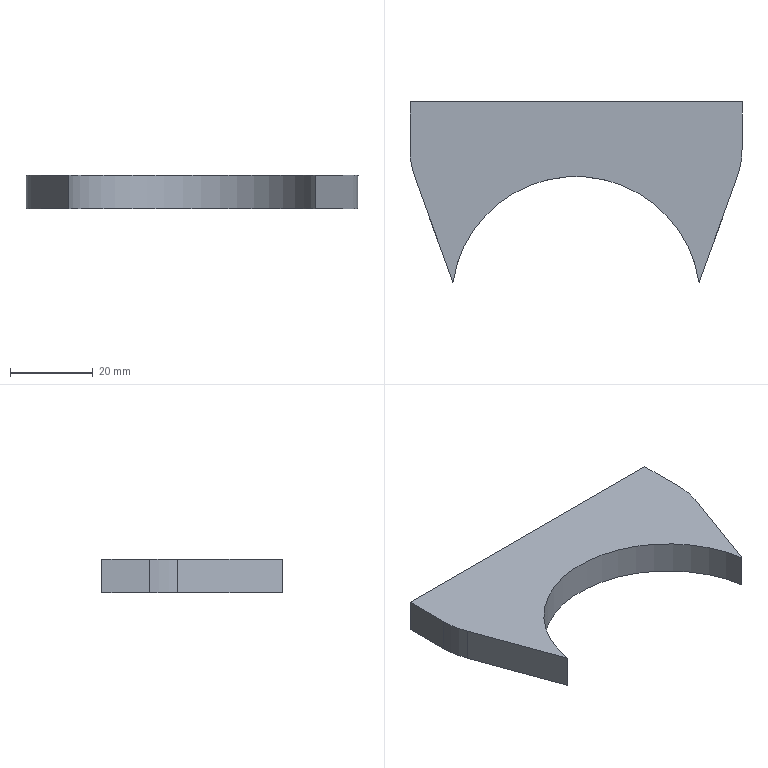Part | SolidWorks | features Fillet 1, FlatPattern 1, SMBaseFlange 1, SheetMetal 1 | 1 solid | 10 faces | box 80 x 43.435 x 8 mm | volume 16306 mm3 | plane 7 | cylinder 3 | commonest cylinder face diameters 40 x2 60 x1
STEP:
#1=CARTESIAN_POINT('',(-40.,48.,-8.));
#2=VERTEX_POINT('',#1);
#3=CARTESIAN_POINT('',(-40.,36.527,-8.));
#4=VERTEX_POINT('',#3);
#5=CARTESIAN_POINT('',(-40.,48.,-8.));
#6=DIRECTION('',(0.,-1.,0.));
#7=VECTOR('',#6,1000.);
#8=LINE('',#5,#7);
#9=EDGE_CURVE('',#2,#4,#8,.T.);
#10=ORIENTED_EDGE('',*,*,#9,.T.);
#11=CARTESIAN_POINT('',(-40.,36.527,0.));
#12=VERTEX_POINT('',#11);
#13=CARTESIAN_POINT('',(-40.,36.527,-8.));
#14=DIRECTION('',(0.,0.,1.));
#15=VECTOR('',#14,1000.);
#16=LINE('',#13,#15);
#17=EDGE_CURVE('',#4,#12,#16,.T.);
#18=ORIENTED_EDGE('',*,*,#17,.T.);
#19=CARTESIAN_POINT('',(-40.,48.,0.));
#20=VERTEX_POINT('',#19);
#21=CARTESIAN_POINT('',(-40.,48.,0.));
#22=DIRECTION('',(0.,-1.,0.));
#23=VECTOR('',#22,1000.);
#24=LINE('',#21,#23);
#25=EDGE_CURVE('',#20,#12,#24,.T.);
#26=ORIENTED_EDGE('',*,*,#25,.F.);
#27=CARTESIAN_POINT('',(-40.,48.,-8.));
#28=DIRECTION('',(0.,0.,1.));
#29=VECTOR('',#28,1000.);
#30=LINE('',#27,#29);
#31=EDGE_CURVE('',#2,#20,#30,.T.);
#32=ORIENTED_EDGE('',*,*,#31,.F.);
#33=EDGE_LOOP('',(#10,#18,#26,#32));
#34=FACE_OUTER_BOUND('',#33,.T.);
#35=CARTESIAN_POINT('',(-40.,48.,-8.));
#36=DIRECTION('',(-1.,0.,0.));
#37=DIRECTION('',(0.,-1.,0.));
#38=AXIS2_PLACEMENT_3D('',#35,#36,#37);
#39=PLANE('',#38);
#40=ADVANCED_FACE('',(#34),#39,.T.);
#41=CARTESIAN_POINT('',(40.,48.,0.));
#42=VERTEX_POINT('',#41);
#43=CARTESIAN_POINT('',(-40.,48.,0.));
#44=DIRECTION('',(-1.,0.,0.));
#45=VECTOR('',#44,1000.);
#46=LINE('',#43,#45);
#47=EDGE_CURVE('',#42,#20,#46,.T.);
#48=ORIENTED_EDGE('',*,*,#47,.F.);
#49=CARTESIAN_POINT('',(40.,48.,-8.));
#50=VERTEX_POINT('',#49);
#51=CARTESIAN_POINT('',(40.,48.,-8.));
#52=DIRECTION('',(0.,0.,1.));
#53=VECTOR('',#52,1000.);
#54=LINE('',#51,#53);
#55=EDGE_CURVE('',#50,#42,#54,.T.);
#56=ORIENTED_EDGE('',*,*,#55,.F.);
#57=CARTESIAN_POINT('',(-40.,48.,-8.));
#58=DIRECTION('',(-1.,0.,0.));
#59=VECTOR('',#58,1000.);
#60=LINE('',#57,#59);
#61=EDGE_CURVE('',#50,#2,#60,.T.);
#62=ORIENTED_EDGE('',*,*,#61,.T.);
#63=ORIENTED_EDGE('',*,*,#31,.T.);
#64=EDGE_LOOP('',(#48,#56,#62,#63));
#65=FACE_OUTER_BOUND('',#64,.T.);
#66=CARTESIAN_POINT('',(-40.,48.,-8.));
#67=DIRECTION('',(0.,1.,0.));
#68=DIRECTION('',(-1.,0.,0.));
#69=AXIS2_PLACEMENT_3D('',#66,#67,#68);
#70=PLANE('',#69);
#71=ADVANCED_FACE('',(#65),#70,.T.);
#72=CARTESIAN_POINT('',(40.,36.527,0.));
#73=VERTEX_POINT('',#72);
#74=CARTESIAN_POINT('',(40.,33.,0.));
#75=DIRECTION('',(0.,1.,0.));
#76=VECTOR('',#75,1000.);
#77=LINE('',#74,#76);
#78=EDGE_CURVE('',#73,#42,#77,.T.);
#79=ORIENTED_EDGE('',*,*,#78,.F.);
#80=CARTESIAN_POINT('',(40.,36.527,-8.));
#81=VERTEX_POINT('',#80);
#82=CARTESIAN_POINT('',(40.,36.527,-8.));
#83=DIRECTION('',(0.,0.,-1.));
#84=VECTOR('',#83,1000.);
#85=LINE('',#82,#84);
#86=EDGE_CURVE('',#73,#81,#85,.T.);
#87=ORIENTED_EDGE('',*,*,#86,.T.);
#88=CARTESIAN_POINT('',(40.,33.,-8.));
#89=DIRECTION('',(0.,1.,0.));
#90=VECTOR('',#89,1000.);
#91=LINE('',#88,#90);
#92=EDGE_CURVE('',#81,#50,#91,.T.);
#93=ORIENTED_EDGE('',*,*,#92,.T.);
#94=ORIENTED_EDGE('',*,*,#55,.T.);
#95=EDGE_LOOP('',(#79,#87,#93,#94));
#96=FACE_OUTER_BOUND('',#95,.T.);
#97=CARTESIAN_POINT('',(40.,33.,-8.));
#98=DIRECTION('',(1.,0.,0.));
#99=DIRECTION('',(0.,1.,0.));
#100=AXIS2_PLACEMENT_3D('',#97,#98,#99);
#101=PLANE('',#100);
#102=ADVANCED_FACE('',(#96),#101,.T.);
#103=CARTESIAN_POINT('',(29.651,4.565,-8.));
#104=VERTEX_POINT('',#103);
#105=CARTESIAN_POINT('',(38.794,29.686,-8.));
#106=VERTEX_POINT('',#105);
#107=CARTESIAN_POINT('',(29.651,4.565,-8.));
#108=DIRECTION('',(0.342,0.9397,0.));
#109=VECTOR('',#108,1000.);
#110=LINE('',#107,#109);
#111=EDGE_CURVE('',#104,#106,#110,.T.);
#112=ORIENTED_EDGE('',*,*,#111,.T.);
#113=CARTESIAN_POINT('',(38.794,29.686,0.));
#114=VERTEX_POINT('',#113);
#115=CARTESIAN_POINT('',(38.794,29.686,-8.));
#116=DIRECTION('',(0.,0.,1.));
#117=VECTOR('',#116,1000.);
#118=LINE('',#115,#117);
#119=EDGE_CURVE('',#106,#114,#118,.T.);
#120=ORIENTED_EDGE('',*,*,#119,.T.);
#121=CARTESIAN_POINT('',(29.651,4.565,0.));
#122=VERTEX_POINT('',#121);
#123=CARTESIAN_POINT('',(29.651,4.565,0.));
#124=DIRECTION('',(0.342,0.9397,0.));
#125=VECTOR('',#124,1000.);
#126=LINE('',#123,#125);
#127=EDGE_CURVE('',#122,#114,#126,.T.);
#128=ORIENTED_EDGE('',*,*,#127,.F.);
#129=CARTESIAN_POINT('',(29.651,4.565,-8.));
#130=DIRECTION('',(0.,0.,1.));
#131=VECTOR('',#130,1000.);
#132=LINE('',#129,#131);
#133=EDGE_CURVE('',#104,#122,#132,.T.);
#134=ORIENTED_EDGE('',*,*,#133,.F.);
#135=EDGE_LOOP('',(#112,#120,#128,#134));
#136=FACE_OUTER_BOUND('',#135,.T.);
#137=CARTESIAN_POINT('',(29.651,4.565,-8.));
#138=DIRECTION('',(0.9397,-0.342,0.));
#139=DIRECTION('',(0.342,0.9397,0.));
#140=AXIS2_PLACEMENT_3D('',#137,#138,#139);
#141=PLANE('',#140);
#142=ADVANCED_FACE('',(#136),#141,.T.);
#143=CARTESIAN_POINT('',(-29.651,4.565,0.));
#144=VERTEX_POINT('',#143);
#145=CARTESIAN_POINT('',(0.,0.,0.));
#146=DIRECTION('',(0.,0.,-1.));
#147=DIRECTION('',(1.,0.,0.));
#148=AXIS2_PLACEMENT_3D('',#145,#146,#147);
#149=CIRCLE('',#148,30.);
#150=EDGE_CURVE('',#144,#122,#149,.T.);
#151=ORIENTED_EDGE('',*,*,#150,.F.);
#152=CARTESIAN_POINT('',(-29.651,4.565,-8.));
#153=VERTEX_POINT('',#152);
#154=CARTESIAN_POINT('',(-29.651,4.565,-8.));
#155=DIRECTION('',(0.,0.,1.));
#156=VECTOR('',#155,1000.);
#157=LINE('',#154,#156);
#158=EDGE_CURVE('',#153,#144,#157,.T.);
#159=ORIENTED_EDGE('',*,*,#158,.F.);
#160=CARTESIAN_POINT('',(0.,0.,-8.));
#161=DIRECTION('',(0.,0.,-1.));
#162=DIRECTION('',(1.,0.,0.));
#163=AXIS2_PLACEMENT_3D('',#160,#161,#162);
#164=CIRCLE('',#163,30.);
#165=EDGE_CURVE('',#153,#104,#164,.T.);
#166=ORIENTED_EDGE('',*,*,#165,.T.);
#167=ORIENTED_EDGE('',*,*,#133,.T.);
#168=EDGE_LOOP('',(#151,#159,#166,#167));
#169=FACE_OUTER_BOUND('',#168,.T.);
#170=CARTESIAN_POINT('',(0.,0.,-8.));
#171=DIRECTION('',(0.,0.,1.));
#172=DIRECTION('',(1.,0.,0.));
#173=AXIS2_PLACEMENT_3D('',#170,#171,#172);
#174=CYLINDRICAL_SURFACE('',#173,30.);
#175=ADVANCED_FACE('',(#169),#174,.F.);
#176=CARTESIAN_POINT('',(-38.794,29.686,0.));
#177=VERTEX_POINT('',#176);
#178=CARTESIAN_POINT('',(-40.,33.,0.));
#179=DIRECTION('',(0.342,-0.9397,0.));
#180=VECTOR('',#179,1000.);
#181=LINE('',#178,#180);
#182=EDGE_CURVE('',#177,#144,#181,.T.);
#183=ORIENTED_EDGE('',*,*,#182,.F.);
#184=CARTESIAN_POINT('',(-38.794,29.686,-8.));
#185=VERTEX_POINT('',#184);
#186=CARTESIAN_POINT('',(-38.794,29.686,-8.));
#187=DIRECTION('',(0.,0.,-1.));
#188=VECTOR('',#187,1000.);
#189=LINE('',#186,#188);
#190=EDGE_CURVE('',#177,#185,#189,.T.);
#191=ORIENTED_EDGE('',*,*,#190,.T.);
#192=CARTESIAN_POINT('',(-40.,33.,-8.));
#193=DIRECTION('',(0.342,-0.9397,0.));
#194=VECTOR('',#193,1000.);
#195=LINE('',#192,#194);
#196=EDGE_CURVE('',#185,#153,#195,.T.);
#197=ORIENTED_EDGE('',*,*,#196,.T.);
#198=ORIENTED_EDGE('',*,*,#158,.T.);
#199=EDGE_LOOP('',(#183,#191,#197,#198));
#200=FACE_OUTER_BOUND('',#199,.T.);
#201=CARTESIAN_POINT('',(-40.,33.,-8.));
#202=DIRECTION('',(-0.9397,-0.342,0.));
#203=DIRECTION('',(0.342,-0.9397,0.));
#204=AXIS2_PLACEMENT_3D('',#201,#202,#203);
#205=PLANE('',#204);
#206=ADVANCED_FACE('',(#200),#205,.T.);
#207=ORIENTED_EDGE('',*,*,#92,.F.);
#208=CARTESIAN_POINT('',(20.,36.527,-8.));
#209=DIRECTION('',(0.,0.,-1.));
#210=DIRECTION('',(1.,0.,0.));
#211=AXIS2_PLACEMENT_3D('',#208,#209,#210);
#212=CIRCLE('',#211,20.);
#213=EDGE_CURVE('',#81,#106,#212,.T.);
#214=ORIENTED_EDGE('',*,*,#213,.T.);
#215=ORIENTED_EDGE('',*,*,#111,.F.);
#216=ORIENTED_EDGE('',*,*,#165,.F.);
#217=ORIENTED_EDGE('',*,*,#196,.F.);
#218=CARTESIAN_POINT('',(-20.,36.527,-8.));
#219=DIRECTION('',(0.,0.,-1.));
#220=DIRECTION('',(1.,0.,0.));
#221=AXIS2_PLACEMENT_3D('',#218,#219,#220);
#222=CIRCLE('',#221,20.);
#223=EDGE_CURVE('',#185,#4,#222,.T.);
#224=ORIENTED_EDGE('',*,*,#223,.T.);
#225=ORIENTED_EDGE('',*,*,#9,.F.);
#226=ORIENTED_EDGE('',*,*,#61,.F.);
#227=EDGE_LOOP('',(#207,#214,#215,#216,#217,#224,#225,#226));
#228=FACE_OUTER_BOUND('',#227,.T.);
#229=CARTESIAN_POINT('',(0.,0.,-8.));
#230=DIRECTION('',(0.,0.,1.));
#231=DIRECTION('',(1.,0.,0.));
#232=AXIS2_PLACEMENT_3D('',#229,#230,#231);
#233=PLANE('',#232);
#234=ADVANCED_FACE('',(#228),#233,.F.);
#235=ORIENTED_EDGE('',*,*,#127,.T.);
#236=CARTESIAN_POINT('',(20.,36.527,0.));
#237=DIRECTION('',(0.,0.,1.));
#238=DIRECTION('',(1.,0.,0.));
#239=AXIS2_PLACEMENT_3D('',#236,#237,#238);
#240=CIRCLE('',#239,20.);
#241=EDGE_CURVE('',#114,#73,#240,.T.);
#242=ORIENTED_EDGE('',*,*,#241,.T.);
#243=ORIENTED_EDGE('',*,*,#78,.T.);
#244=ORIENTED_EDGE('',*,*,#47,.T.);
#245=ORIENTED_EDGE('',*,*,#25,.T.);
#246=CARTESIAN_POINT('',(-20.,36.527,0.));
#247=DIRECTION('',(0.,0.,1.));
#248=DIRECTION('',(1.,0.,0.));
#249=AXIS2_PLACEMENT_3D('',#246,#247,#248);
#250=CIRCLE('',#249,20.);
#251=EDGE_CURVE('',#12,#177,#250,.T.);
#252=ORIENTED_EDGE('',*,*,#251,.T.);
#253=ORIENTED_EDGE('',*,*,#182,.T.);
#254=ORIENTED_EDGE('',*,*,#150,.T.);
#255=EDGE_LOOP('',(#235,#242,#243,#244,#245,#252,#253,#254));
#256=FACE_OUTER_BOUND('',#255,.T.);
#257=CARTESIAN_POINT('',(0.,0.,0.));
#258=DIRECTION('',(0.,0.,1.));
#259=DIRECTION('',(1.,0.,0.));
#260=AXIS2_PLACEMENT_3D('',#257,#258,#259);
#261=PLANE('',#260);
#262=ADVANCED_FACE('',(#256),#261,.T.);
#263=ORIENTED_EDGE('',*,*,#213,.F.);
#264=ORIENTED_EDGE('',*,*,#86,.F.);
#265=ORIENTED_EDGE('',*,*,#241,.F.);
#266=ORIENTED_EDGE('',*,*,#119,.F.);
#267=EDGE_LOOP('',(#263,#264,#265,#266));
#268=FACE_OUTER_BOUND('',#267,.T.);
#269=CARTESIAN_POINT('',(20.,36.527,-8.));
#270=DIRECTION('',(0.,0.,1.));
#271=DIRECTION('',(1.,0.,0.));
#272=AXIS2_PLACEMENT_3D('',#269,#270,#271);
#273=CYLINDRICAL_SURFACE('',#272,20.);
#274=ADVANCED_FACE('',(#268),#273,.T.);
#275=ORIENTED_EDGE('',*,*,#223,.F.);
#276=ORIENTED_EDGE('',*,*,#190,.F.);
#277=ORIENTED_EDGE('',*,*,#251,.F.);
#278=ORIENTED_EDGE('',*,*,#17,.F.);
#279=EDGE_LOOP('',(#275,#276,#277,#278));
#280=FACE_OUTER_BOUND('',#279,.T.);
#281=CARTESIAN_POINT('',(-20.,36.527,-8.));
#282=DIRECTION('',(0.,0.,1.));
#283=DIRECTION('',(1.,0.,0.));
#284=AXIS2_PLACEMENT_3D('',#281,#282,#283);
#285=CYLINDRICAL_SURFACE('',#284,20.);
#286=ADVANCED_FACE('',(#280),#285,.T.);
#287=CLOSED_SHELL('',(#40,#71,#102,#142,#175,#206,#234,#262,#274,#286));
#288=MANIFOLD_SOLID_BREP('',#287);
#289=CARTESIAN_POINT('',(0.,0.,0.));
#290=DIRECTION('',(0.,0.,1.));
#291=DIRECTION('',(1.,0.,0.));
#292=AXIS2_PLACEMENT_3D('',#289,#290,#291);
#293=(LENGTH_UNIT()NAMED_UNIT(*)SI_UNIT(.MILLI.,.METRE.));
#294=UNCERTAINTY_MEASURE_WITH_UNIT(LENGTH_MEASURE(0.00001),#293,'','');
#295=(NAMED_UNIT(*)PLANE_ANGLE_UNIT()SI_UNIT($,.RADIAN.));
#296=(NAMED_UNIT(*)SI_UNIT($,.STERADIAN.)SOLID_ANGLE_UNIT());
#297=(GEOMETRIC_REPRESENTATION_CONTEXT(3)GLOBAL_UNCERTAINTY_ASSIGNED_CONTEXT((#294))GLOBAL_UNIT_ASSIGNED_CONTEXT((#293,#295,#296))REPRESENTATION_CONTEXT('',''));
#298=ADVANCED_BREP_SHAPE_REPRESENTATION('',(#288,#292),#297);